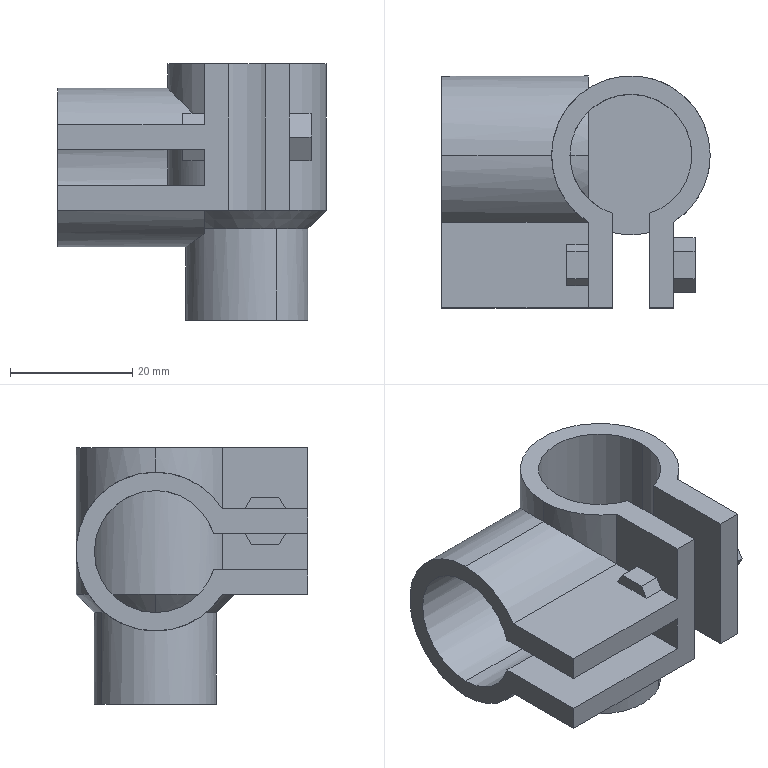Part | SolidWorks | features MBimport 1 | 1 solid | 59 faces | box 44 x 38 x 42 mm | volume 20383 mm3 | plane 35 | cylinder 20 | cone 4 | commonest cylinder face diameters 20 x11 26 x9